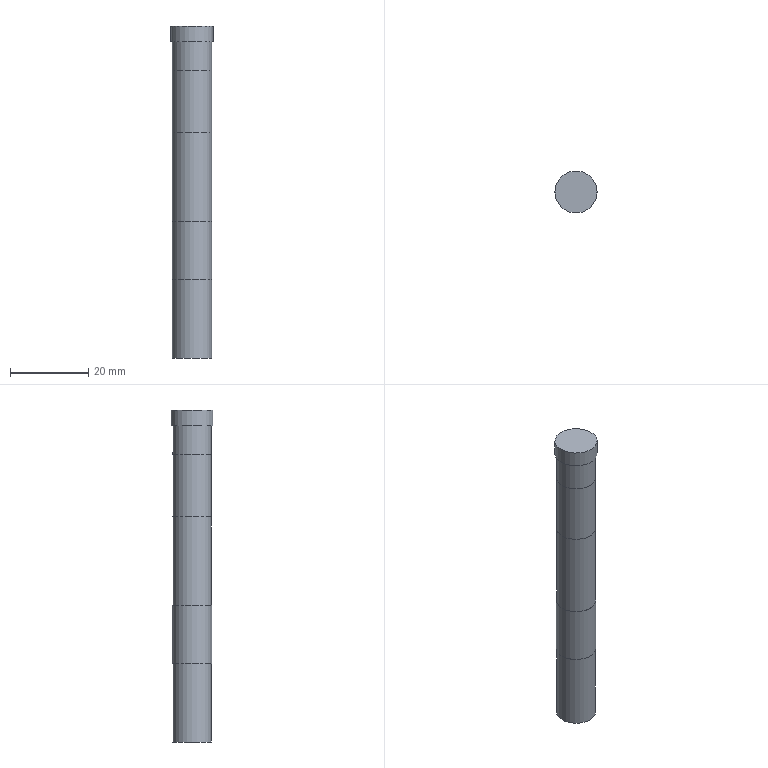Part | NX | features BREP 2 | 2 solids | 14 faces | box 10.8 x 10.8 x 85 mm | volume 8276 mm3 | plane 7 | cylinder 5 | torus 1 | cone 1 | commonest cylinder face diameters 10 x2 10.008 x1 10.1 x1 10.8 x1
STEP:
#1=CARTESIAN_POINT('',(5.004,0.,37.667));
#2=VERTEX_POINT('',#1);
#3=CARTESIAN_POINT('',(0.,0.,37.667));
#4=DIRECTION('',(0.,0.,1.));
#5=DIRECTION('',(1.,0.,0.));
#6=AXIS2_PLACEMENT_3D('',#3,#4,#5);
#7=CIRCLE('',#6,5.004);
#8=EDGE_CURVE('',#2,#2,#7,.T.);
#9=ORIENTED_EDGE('',*,*,#8,.T.);
#10=EDGE_LOOP('',(#9));
#11=FACE_BOUND('',#10,.T.);
#12=CARTESIAN_POINT('',(5.004,0.,53.5));
#13=VERTEX_POINT('',#12);
#14=CARTESIAN_POINT('',(0.,0.,53.5));
#15=DIRECTION('',(0.,0.,-1.));
#16=DIRECTION('',(1.,0.,0.));
#17=AXIS2_PLACEMENT_3D('',#14,#15,#16);
#18=CIRCLE('',#17,5.004);
#19=EDGE_CURVE('',#13,#13,#18,.T.);
#20=ORIENTED_EDGE('',*,*,#19,.T.);
#21=EDGE_LOOP('',(#20));
#22=FACE_BOUND('',#21,.T.);
#23=CARTESIAN_POINT('',(0.,0.,36.));
#24=DIRECTION('',(0.,0.,1.));
#25=DIRECTION('',(-1.,0.,0.));
#26=AXIS2_PLACEMENT_3D('',#23,#24,#25);
#27=CYLINDRICAL_SURFACE('',#26,5.004);
#28=ADVANCED_FACE('',(#11,#22),#27,.T.);
#29=CARTESIAN_POINT('',(4.557,0.,36.));
#30=VERTEX_POINT('',#29);
#31=CARTESIAN_POINT('',(0.,0.,36.));
#32=DIRECTION('',(0.,0.,-1.));
#33=DIRECTION('',(1.,0.,0.));
#34=AXIS2_PLACEMENT_3D('',#31,#32,#33);
#35=CIRCLE('',#34,4.557);
#36=EDGE_CURVE('',#30,#30,#35,.T.);
#37=ORIENTED_EDGE('',*,*,#36,.T.);
#38=EDGE_LOOP('',(#37));
#39=FACE_BOUND('',#38,.T.);
#40=CARTESIAN_POINT('',(0.,0.,36.));
#41=DIRECTION('',(0.,0.,1.));
#42=DIRECTION('',(-1.,0.,0.));
#43=AXIS2_PLACEMENT_3D('',#40,#41,#42);
#44=PLANE('',#43);
#45=ADVANCED_FACE('',(#39),#44,.F.);
#46=CARTESIAN_POINT('',(2.504,0.,56.));
#47=VERTEX_POINT('',#46);
#48=CARTESIAN_POINT('',(0.,0.,56.));
#49=DIRECTION('',(0.,0.,1.));
#50=DIRECTION('',(1.,0.,0.));
#51=AXIS2_PLACEMENT_3D('',#48,#49,#50);
#52=CIRCLE('',#51,2.504);
#53=EDGE_CURVE('',#47,#47,#52,.T.);
#54=ORIENTED_EDGE('',*,*,#53,.T.);
#55=EDGE_LOOP('',(#54));
#56=FACE_BOUND('',#55,.T.);
#57=CARTESIAN_POINT('',(0.,0.,56.));
#58=DIRECTION('',(0.,0.,1.));
#59=DIRECTION('',(-1.,0.,0.));
#60=AXIS2_PLACEMENT_3D('',#57,#58,#59);
#61=PLANE('',#60);
#62=ADVANCED_FACE('',(#56),#61,.T.);
#63=ORIENTED_EDGE('',*,*,#19,.F.);
#64=EDGE_LOOP('',(#63));
#65=FACE_BOUND('',#64,.T.);
#66=ORIENTED_EDGE('',*,*,#53,.F.);
#67=EDGE_LOOP('',(#66));
#68=FACE_BOUND('',#67,.T.);
#69=CARTESIAN_POINT('',(0.,0.,53.5));
#70=DIRECTION('',(0.,0.,1.));
#71=DIRECTION('',(-1.,0.,0.));
#72=AXIS2_PLACEMENT_3D('',#69,#70,#71);
#73=TOROIDAL_SURFACE('',#72,2.504,2.5);
#74=ADVANCED_FACE('',(#65,#68),#73,.T.);
#75=ORIENTED_EDGE('',*,*,#36,.F.);
#76=EDGE_LOOP('',(#75));
#77=FACE_BOUND('',#76,.T.);
#78=ORIENTED_EDGE('',*,*,#8,.F.);
#79=EDGE_LOOP('',(#78));
#80=FACE_BOUND('',#79,.T.);
#81=CARTESIAN_POINT('',(0.,0.,37.667));
#82=DIRECTION('',(0.,0.,1.));
#83=DIRECTION('',(-1.,0.,0.));
#84=AXIS2_PLACEMENT_3D('',#81,#82,#83);
#85=CONICAL_SURFACE('',#84,5.004,0.2618);
#86=ADVANCED_FACE('',(#77,#80),#85,.T.);
#87=CLOSED_SHELL('',(#28,#45,#62,#74,#86));
#88=MANIFOLD_SOLID_BREP('',#87);
#89=CARTESIAN_POINT('',(5.4,0.,61.));
#90=VERTEX_POINT('',#89);
#91=CARTESIAN_POINT('',(0.,0.,61.));
#92=DIRECTION('',(0.,0.,1.));
#93=DIRECTION('',(1.,0.,0.));
#94=AXIS2_PLACEMENT_3D('',#91,#92,#93);
#95=CIRCLE('',#94,5.4);
#96=EDGE_CURVE('',#90,#90,#95,.T.);
#97=ORIENTED_EDGE('',*,*,#96,.T.);
#98=EDGE_LOOP('',(#97));
#99=FACE_BOUND('',#98,.T.);
#100=CARTESIAN_POINT('',(5.4,0.,65.));
#101=VERTEX_POINT('',#100);
#102=CARTESIAN_POINT('',(0.,0.,65.));
#103=DIRECTION('',(0.,0.,1.));
#104=DIRECTION('',(1.,0.,0.));
#105=AXIS2_PLACEMENT_3D('',#102,#103,#104);
#106=CIRCLE('',#105,5.4);
#107=EDGE_CURVE('',#101,#101,#106,.T.);
#108=ORIENTED_EDGE('',*,*,#107,.F.);
#109=EDGE_LOOP('',(#108));
#110=FACE_BOUND('',#109,.T.);
#111=CARTESIAN_POINT('',(0.,0.,61.));
#112=DIRECTION('',(0.,0.,1.));
#113=DIRECTION('',(-1.,0.,0.));
#114=AXIS2_PLACEMENT_3D('',#111,#112,#113);
#115=CYLINDRICAL_SURFACE('',#114,5.4);
#116=ADVANCED_FACE('',(#99,#110),#115,.T.);
#117=CARTESIAN_POINT('',(-5.,0.,61.));
#118=VERTEX_POINT('',#117);
#119=CARTESIAN_POINT('',(0.,0.,61.));
#120=DIRECTION('',(0.,0.,-1.));
#121=DIRECTION('',(-1.,0.,0.));
#122=AXIS2_PLACEMENT_3D('',#119,#120,#121);
#123=CIRCLE('',#122,5.);
#124=EDGE_CURVE('',#118,#118,#123,.T.);
#125=ORIENTED_EDGE('',*,*,#124,.F.);
#126=EDGE_LOOP('',(#125));
#127=FACE_BOUND('',#126,.T.);
#128=ORIENTED_EDGE('',*,*,#96,.F.);
#129=EDGE_LOOP('',(#128));
#130=FACE_BOUND('',#129,.T.);
#131=CARTESIAN_POINT('',(0.,0.,61.));
#132=DIRECTION('',(0.,0.,1.));
#133=DIRECTION('',(-1.,0.,0.));
#134=AXIS2_PLACEMENT_3D('',#131,#132,#133);
#135=PLANE('',#134);
#136=ADVANCED_FACE('',(#127,#130),#135,.F.);
#137=ORIENTED_EDGE('',*,*,#107,.T.);
#138=EDGE_LOOP('',(#137));
#139=FACE_BOUND('',#138,.T.);
#140=CARTESIAN_POINT('',(0.,0.,65.));
#141=DIRECTION('',(0.,0.,1.));
#142=DIRECTION('',(-1.,0.,0.));
#143=AXIS2_PLACEMENT_3D('',#140,#141,#142);
#144=PLANE('',#143);
#145=ADVANCED_FACE('',(#139),#144,.T.);
#146=CARTESIAN_POINT('',(-5.,0.,15.));
#147=VERTEX_POINT('',#146);
#148=CARTESIAN_POINT('',(0.,0.,15.));
#149=DIRECTION('',(0.,0.,-1.));
#150=DIRECTION('',(-1.,0.,0.));
#151=AXIS2_PLACEMENT_3D('',#148,#149,#150);
#152=CIRCLE('',#151,5.);
#153=EDGE_CURVE('',#147,#147,#152,.T.);
#154=ORIENTED_EDGE('',*,*,#153,.F.);
#155=EDGE_LOOP('',(#154));
#156=FACE_BOUND('',#155,.T.);
#157=ORIENTED_EDGE('',*,*,#124,.T.);
#158=EDGE_LOOP('',(#157));
#159=FACE_BOUND('',#158,.T.);
#160=CARTESIAN_POINT('',(0.,0.,61.));
#161=DIRECTION('',(0.,0.,-1.));
#162=DIRECTION('',(1.,0.,0.));
#163=AXIS2_PLACEMENT_3D('',#160,#161,#162);
#164=CYLINDRICAL_SURFACE('',#163,5.);
#165=ADVANCED_FACE('',(#156,#159),#164,.T.);
#166=CARTESIAN_POINT('',(-5.,0.,0.));
#167=VERTEX_POINT('',#166);
#168=CARTESIAN_POINT('',(0.,0.,0.));
#169=DIRECTION('',(0.,0.,-1.));
#170=DIRECTION('',(-1.,0.,0.));
#171=AXIS2_PLACEMENT_3D('',#168,#169,#170);
#172=CIRCLE('',#171,5.);
#173=EDGE_CURVE('',#167,#167,#172,.T.);
#174=ORIENTED_EDGE('',*,*,#173,.F.);
#175=EDGE_LOOP('',(#174));
#176=FACE_BOUND('',#175,.T.);
#177=CARTESIAN_POINT('',(-5.05,0.,0.));
#178=VERTEX_POINT('',#177);
#179=CARTESIAN_POINT('',(0.,0.,0.));
#180=DIRECTION('',(0.,0.,-1.));
#181=DIRECTION('',(-1.,0.,0.));
#182=AXIS2_PLACEMENT_3D('',#179,#180,#181);
#183=CIRCLE('',#182,5.05);
#184=EDGE_CURVE('',#178,#178,#183,.T.);
#185=ORIENTED_EDGE('',*,*,#184,.T.);
#186=EDGE_LOOP('',(#185));
#187=FACE_BOUND('',#186,.T.);
#188=CARTESIAN_POINT('',(0.,0.,0.));
#189=DIRECTION('',(0.,0.,-1.));
#190=DIRECTION('',(1.,0.,0.));
#191=AXIS2_PLACEMENT_3D('',#188,#189,#190);
#192=PLANE('',#191);
#193=ADVANCED_FACE('',(#176,#187),#192,.T.);
#194=ORIENTED_EDGE('',*,*,#153,.T.);
#195=EDGE_LOOP('',(#194));
#196=FACE_BOUND('',#195,.T.);
#197=CARTESIAN_POINT('',(-5.05,0.,15.));
#198=VERTEX_POINT('',#197);
#199=CARTESIAN_POINT('',(0.,0.,15.));
#200=DIRECTION('',(0.,0.,-1.));
#201=DIRECTION('',(-1.,0.,0.));
#202=AXIS2_PLACEMENT_3D('',#199,#200,#201);
#203=CIRCLE('',#202,5.05);
#204=EDGE_CURVE('',#198,#198,#203,.T.);
#205=ORIENTED_EDGE('',*,*,#204,.F.);
#206=EDGE_LOOP('',(#205));
#207=FACE_BOUND('',#206,.T.);
#208=CARTESIAN_POINT('',(0.,0.,15.));
#209=DIRECTION('',(0.,0.,1.));
#210=DIRECTION('',(-1.,0.,0.));
#211=AXIS2_PLACEMENT_3D('',#208,#209,#210);
#212=PLANE('',#211);
#213=ADVANCED_FACE('',(#196,#207),#212,.T.);
#214=ORIENTED_EDGE('',*,*,#184,.F.);
#215=EDGE_LOOP('',(#214));
#216=FACE_BOUND('',#215,.T.);
#217=ORIENTED_EDGE('',*,*,#204,.T.);
#218=EDGE_LOOP('',(#217));
#219=FACE_BOUND('',#218,.T.);
#220=CARTESIAN_POINT('',(0.,0.,15.));
#221=DIRECTION('',(0.,0.,-1.));
#222=DIRECTION('',(1.,0.,0.));
#223=AXIS2_PLACEMENT_3D('',#220,#221,#222);
#224=CYLINDRICAL_SURFACE('',#223,5.05);
#225=ADVANCED_FACE('',(#216,#219),#224,.T.);
#226=CARTESIAN_POINT('',(-5.,0.,-20.));
#227=VERTEX_POINT('',#226);
#228=CARTESIAN_POINT('',(0.,0.,-20.));
#229=DIRECTION('',(0.,0.,-1.));
#230=DIRECTION('',(-1.,0.,0.));
#231=AXIS2_PLACEMENT_3D('',#228,#229,#230);
#232=CIRCLE('',#231,5.);
#233=EDGE_CURVE('',#227,#227,#232,.T.);
#234=ORIENTED_EDGE('',*,*,#233,.T.);
#235=EDGE_LOOP('',(#234));
#236=FACE_BOUND('',#235,.T.);
#237=CARTESIAN_POINT('',(0.,0.,-20.));
#238=DIRECTION('',(0.,0.,-1.));
#239=DIRECTION('',(1.,0.,0.));
#240=AXIS2_PLACEMENT_3D('',#237,#238,#239);
#241=PLANE('',#240);
#242=ADVANCED_FACE('',(#236),#241,.T.);
#243=ORIENTED_EDGE('',*,*,#233,.F.);
#244=EDGE_LOOP('',(#243));
#245=FACE_BOUND('',#244,.T.);
#246=ORIENTED_EDGE('',*,*,#173,.T.);
#247=EDGE_LOOP('',(#246));
#248=FACE_BOUND('',#247,.T.);
#249=CARTESIAN_POINT('',(0.,0.,0.));
#250=DIRECTION('',(0.,0.,-1.));
#251=DIRECTION('',(1.,0.,0.));
#252=AXIS2_PLACEMENT_3D('',#249,#250,#251);
#253=CYLINDRICAL_SURFACE('',#252,5.);
#254=ADVANCED_FACE('',(#245,#248),#253,.T.);
#255=CLOSED_SHELL('',(#116,#136,#145,#165,#193,#213,#225,#242,#254));
#256=MANIFOLD_SOLID_BREP('',#255);
#257=(LENGTH_UNIT()NAMED_UNIT(*)SI_UNIT(.MILLI.,.METRE.));
#258=UNCERTAINTY_MEASURE_WITH_UNIT(LENGTH_MEASURE(0.00001),#257,'','');
#259=(NAMED_UNIT(*)PLANE_ANGLE_UNIT()SI_UNIT($,.RADIAN.));
#260=(NAMED_UNIT(*)SI_UNIT($,.STERADIAN.)SOLID_ANGLE_UNIT());
#261=(GEOMETRIC_REPRESENTATION_CONTEXT(3)GLOBAL_UNCERTAINTY_ASSIGNED_CONTEXT((#258))GLOBAL_UNIT_ASSIGNED_CONTEXT((#257,#259,#260))REPRESENTATION_CONTEXT('',''));
#262=ADVANCED_BREP_SHAPE_REPRESENTATION('',(#88,#256),#261);